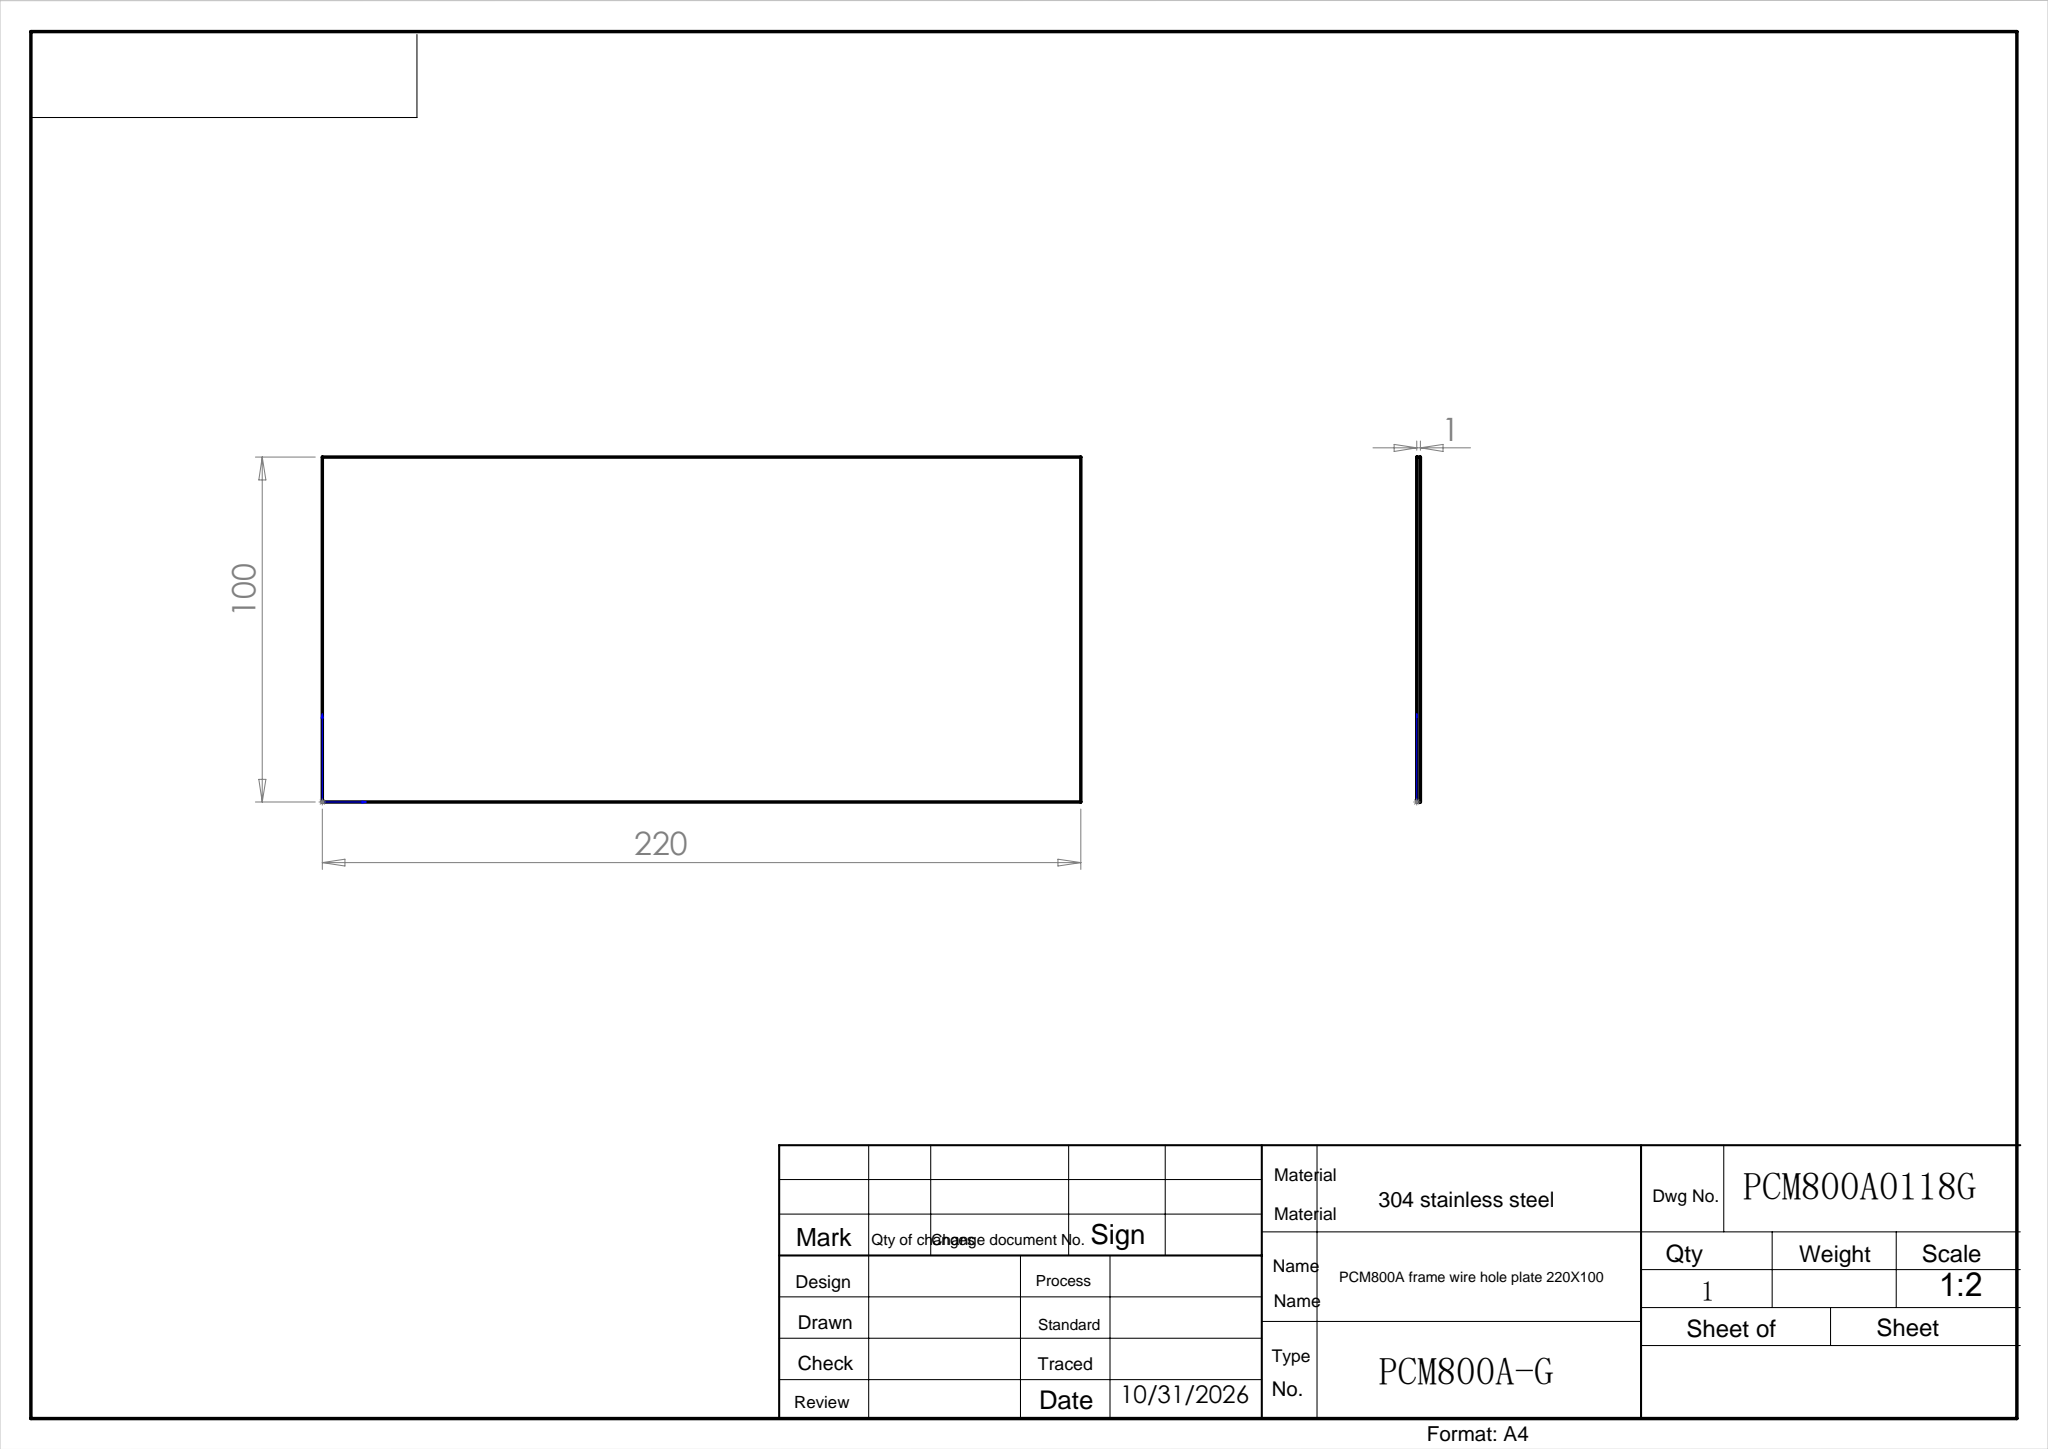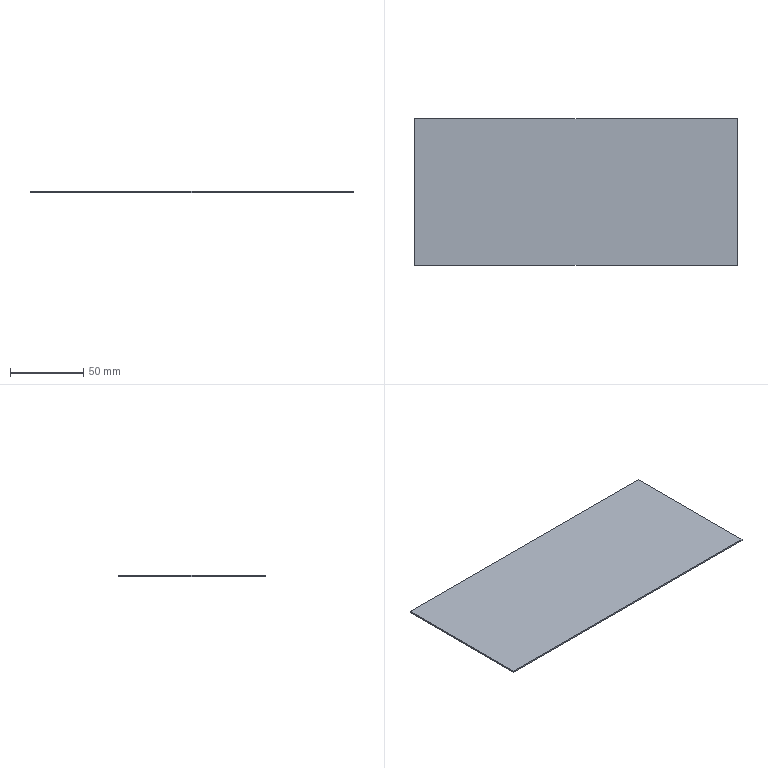Part | SolidWorks | features Extrusion 1 | 1 solid | 6 faces | box 220 x 100 x 1 mm | volume 22000 mm3 | plane 6
STEP:
#1=CARTESIAN_POINT('',(0.,100.,0.));
#2=VERTEX_POINT('',#1);
#3=CARTESIAN_POINT('',(0.,0.,0.));
#4=VERTEX_POINT('',#3);
#5=CARTESIAN_POINT('',(0.,0.,0.));
#6=DIRECTION('',(0.,-1.,0.));
#7=VECTOR('',#6,1000.);
#8=LINE('',#5,#7);
#9=EDGE_CURVE('',#2,#4,#8,.T.);
#10=ORIENTED_EDGE('',*,*,#9,.T.);
#11=CARTESIAN_POINT('',(0.,0.,1.));
#12=VERTEX_POINT('',#11);
#13=CARTESIAN_POINT('',(0.,0.,1.));
#14=DIRECTION('',(0.,0.,-1.));
#15=VECTOR('',#14,1000.);
#16=LINE('',#13,#15);
#17=EDGE_CURVE('',#12,#4,#16,.T.);
#18=ORIENTED_EDGE('',*,*,#17,.F.);
#19=CARTESIAN_POINT('',(0.,100.,1.));
#20=VERTEX_POINT('',#19);
#21=CARTESIAN_POINT('',(0.,0.,1.));
#22=DIRECTION('',(0.,-1.,0.));
#23=VECTOR('',#22,1000.);
#24=LINE('',#21,#23);
#25=EDGE_CURVE('',#20,#12,#24,.T.);
#26=ORIENTED_EDGE('',*,*,#25,.F.);
#27=CARTESIAN_POINT('',(0.,100.,1.));
#28=DIRECTION('',(0.,0.,-1.));
#29=VECTOR('',#28,1000.);
#30=LINE('',#27,#29);
#31=EDGE_CURVE('',#20,#2,#30,.T.);
#32=ORIENTED_EDGE('',*,*,#31,.T.);
#33=EDGE_LOOP('',(#10,#18,#26,#32));
#34=FACE_OUTER_BOUND('',#33,.T.);
#35=CARTESIAN_POINT('',(0.,0.,1.));
#36=DIRECTION('',(1.,0.,0.));
#37=DIRECTION('',(0.,1.,0.));
#38=AXIS2_PLACEMENT_3D('',#35,#36,#37);
#39=PLANE('',#38);
#40=ADVANCED_FACE('',(#34),#39,.F.);
#41=CARTESIAN_POINT('',(220.,0.,0.));
#42=VERTEX_POINT('',#41);
#43=CARTESIAN_POINT('',(0.,0.,0.));
#44=DIRECTION('',(1.,0.,0.));
#45=VECTOR('',#44,1000.);
#46=LINE('',#43,#45);
#47=EDGE_CURVE('',#4,#42,#46,.T.);
#48=ORIENTED_EDGE('',*,*,#47,.T.);
#49=CARTESIAN_POINT('',(220.,0.,1.));
#50=VERTEX_POINT('',#49);
#51=CARTESIAN_POINT('',(220.,0.,1.));
#52=DIRECTION('',(0.,0.,-1.));
#53=VECTOR('',#52,1000.);
#54=LINE('',#51,#53);
#55=EDGE_CURVE('',#50,#42,#54,.T.);
#56=ORIENTED_EDGE('',*,*,#55,.F.);
#57=CARTESIAN_POINT('',(0.,0.,1.));
#58=DIRECTION('',(1.,0.,0.));
#59=VECTOR('',#58,1000.);
#60=LINE('',#57,#59);
#61=EDGE_CURVE('',#12,#50,#60,.T.);
#62=ORIENTED_EDGE('',*,*,#61,.F.);
#63=ORIENTED_EDGE('',*,*,#17,.T.);
#64=EDGE_LOOP('',(#48,#56,#62,#63));
#65=FACE_OUTER_BOUND('',#64,.T.);
#66=CARTESIAN_POINT('',(0.,0.,1.));
#67=DIRECTION('',(0.,1.,0.));
#68=DIRECTION('',(0.,0.,1.));
#69=AXIS2_PLACEMENT_3D('',#66,#67,#68);
#70=PLANE('',#69);
#71=ADVANCED_FACE('',(#65),#70,.F.);
#72=CARTESIAN_POINT('',(220.,100.,0.));
#73=VERTEX_POINT('',#72);
#74=CARTESIAN_POINT('',(220.,0.,0.));
#75=DIRECTION('',(0.,1.,0.));
#76=VECTOR('',#75,1000.);
#77=LINE('',#74,#76);
#78=EDGE_CURVE('',#42,#73,#77,.T.);
#79=ORIENTED_EDGE('',*,*,#78,.T.);
#80=CARTESIAN_POINT('',(220.,100.,1.));
#81=VERTEX_POINT('',#80);
#82=CARTESIAN_POINT('',(220.,100.,1.));
#83=DIRECTION('',(0.,0.,-1.));
#84=VECTOR('',#83,1000.);
#85=LINE('',#82,#84);
#86=EDGE_CURVE('',#81,#73,#85,.T.);
#87=ORIENTED_EDGE('',*,*,#86,.F.);
#88=CARTESIAN_POINT('',(220.,0.,1.));
#89=DIRECTION('',(0.,1.,0.));
#90=VECTOR('',#89,1000.);
#91=LINE('',#88,#90);
#92=EDGE_CURVE('',#50,#81,#91,.T.);
#93=ORIENTED_EDGE('',*,*,#92,.F.);
#94=ORIENTED_EDGE('',*,*,#55,.T.);
#95=EDGE_LOOP('',(#79,#87,#93,#94));
#96=FACE_OUTER_BOUND('',#95,.T.);
#97=CARTESIAN_POINT('',(220.,0.,1.));
#98=DIRECTION('',(-1.,0.,0.));
#99=DIRECTION('',(0.,0.,1.));
#100=AXIS2_PLACEMENT_3D('',#97,#98,#99);
#101=PLANE('',#100);
#102=ADVANCED_FACE('',(#96),#101,.F.);
#103=CARTESIAN_POINT('',(0.,100.,0.));
#104=DIRECTION('',(-1.,0.,0.));
#105=VECTOR('',#104,1000.);
#106=LINE('',#103,#105);
#107=EDGE_CURVE('',#73,#2,#106,.T.);
#108=ORIENTED_EDGE('',*,*,#107,.T.);
#109=ORIENTED_EDGE('',*,*,#31,.F.);
#110=CARTESIAN_POINT('',(0.,100.,1.));
#111=DIRECTION('',(-1.,0.,0.));
#112=VECTOR('',#111,1000.);
#113=LINE('',#110,#112);
#114=EDGE_CURVE('',#81,#20,#113,.T.);
#115=ORIENTED_EDGE('',*,*,#114,.F.);
#116=ORIENTED_EDGE('',*,*,#86,.T.);
#117=EDGE_LOOP('',(#108,#109,#115,#116));
#118=FACE_OUTER_BOUND('',#117,.T.);
#119=CARTESIAN_POINT('',(0.,100.,1.));
#120=DIRECTION('',(0.,-1.,0.));
#121=DIRECTION('',(0.,0.,-1.));
#122=AXIS2_PLACEMENT_3D('',#119,#120,#121);
#123=PLANE('',#122);
#124=ADVANCED_FACE('',(#118),#123,.F.);
#125=ORIENTED_EDGE('',*,*,#25,.T.);
#126=ORIENTED_EDGE('',*,*,#61,.T.);
#127=ORIENTED_EDGE('',*,*,#92,.T.);
#128=ORIENTED_EDGE('',*,*,#114,.T.);
#129=EDGE_LOOP('',(#125,#126,#127,#128));
#130=FACE_OUTER_BOUND('',#129,.T.);
#131=CARTESIAN_POINT('',(0.,100.,1.));
#132=DIRECTION('',(0.,0.,-1.));
#133=DIRECTION('',(-1.,0.,0.));
#134=AXIS2_PLACEMENT_3D('',#131,#132,#133);
#135=PLANE('',#134);
#136=ADVANCED_FACE('',(#130),#135,.F.);
#137=ORIENTED_EDGE('',*,*,#9,.F.);
#138=ORIENTED_EDGE('',*,*,#107,.F.);
#139=ORIENTED_EDGE('',*,*,#78,.F.);
#140=ORIENTED_EDGE('',*,*,#47,.F.);
#141=EDGE_LOOP('',(#137,#138,#139,#140));
#142=FACE_OUTER_BOUND('',#141,.T.);
#143=CARTESIAN_POINT('',(0.,100.,0.));
#144=DIRECTION('',(0.,0.,-1.));
#145=DIRECTION('',(-1.,0.,0.));
#146=AXIS2_PLACEMENT_3D('',#143,#144,#145);
#147=PLANE('',#146);
#148=ADVANCED_FACE('',(#142),#147,.T.);
#149=CLOSED_SHELL('',(#40,#71,#102,#124,#136,#148));
#150=MANIFOLD_SOLID_BREP('',#149);
#151=CARTESIAN_POINT('',(0.,0.,0.));
#152=DIRECTION('',(0.,0.,1.));
#153=DIRECTION('',(1.,0.,0.));
#154=AXIS2_PLACEMENT_3D('',#151,#152,#153);
#155=(LENGTH_UNIT()NAMED_UNIT(*)SI_UNIT(.MILLI.,.METRE.));
#156=UNCERTAINTY_MEASURE_WITH_UNIT(LENGTH_MEASURE(0.00001),#155,'','');
#157=(NAMED_UNIT(*)PLANE_ANGLE_UNIT()SI_UNIT($,.RADIAN.));
#158=(NAMED_UNIT(*)SI_UNIT($,.STERADIAN.)SOLID_ANGLE_UNIT());
#159=(GEOMETRIC_REPRESENTATION_CONTEXT(3)GLOBAL_UNCERTAINTY_ASSIGNED_CONTEXT((#156))GLOBAL_UNIT_ASSIGNED_CONTEXT((#155,#157,#158))REPRESENTATION_CONTEXT('',''));
#160=ADVANCED_BREP_SHAPE_REPRESENTATION('',(#150,#154),#159);